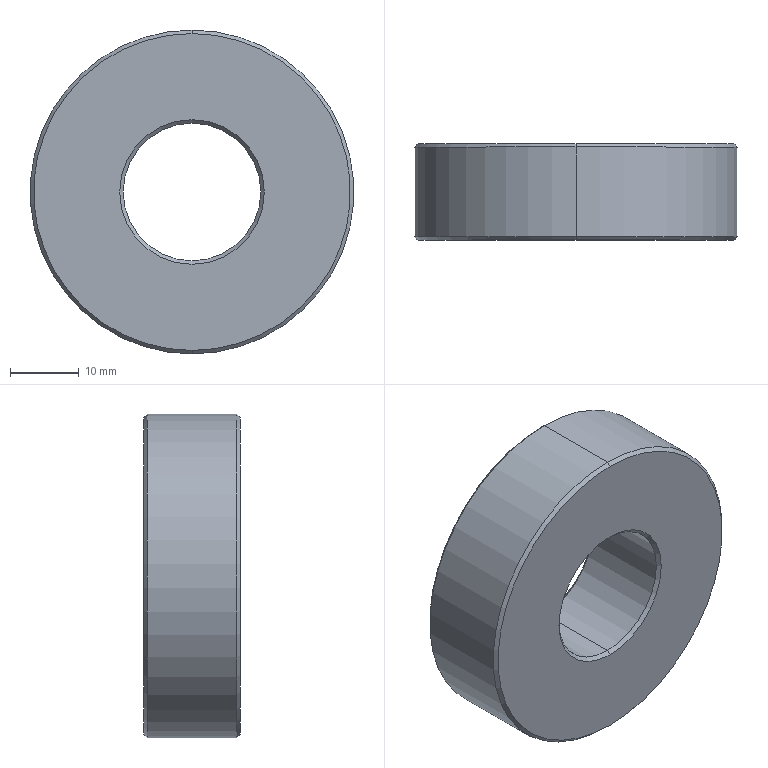Part | SolidWorks | features Chamfer 1, Extrusion 1 | 1 solid | 14 faces | box 47 x 14 x 47 mm | volume 19838 mm3 | cone 8 | cylinder 4 | plane 2 | commonest cylinder face diameters 20 x2 47 x2
STEP:
#1=CARTESIAN_POINT('',(0.,13.5,-10.));
#2=VERTEX_POINT('',#1);
#3=CARTESIAN_POINT('',(0.,13.5,10.));
#4=VERTEX_POINT('',#3);
#5=CARTESIAN_POINT('',(0.,13.5,0.));
#6=DIRECTION('',(0.,1.,0.));
#7=DIRECTION('',(0.,0.,1.));
#8=AXIS2_PLACEMENT_3D('',#5,#6,#7);
#9=CIRCLE('',#8,10.);
#10=EDGE_CURVE('',#2,#4,#9,.T.);
#11=ORIENTED_EDGE('',*,*,#10,.F.);
#12=CARTESIAN_POINT('',(0.,14.,-10.5));
#13=VERTEX_POINT('',#12);
#14=CARTESIAN_POINT('',(0.,13.5,-10.));
#15=DIRECTION('',(0.,0.7071,-0.7071));
#16=VECTOR('',#15,1000.);
#17=LINE('',#14,#16);
#18=EDGE_CURVE('',#2,#13,#17,.T.);
#19=ORIENTED_EDGE('',*,*,#18,.T.);
#20=CARTESIAN_POINT('',(0.,14.,10.5));
#21=VERTEX_POINT('',#20);
#22=CARTESIAN_POINT('',(0.,14.,0.));
#23=DIRECTION('',(0.,-1.,0.));
#24=DIRECTION('',(0.,0.,1.));
#25=AXIS2_PLACEMENT_3D('',#22,#23,#24);
#26=CIRCLE('',#25,10.5);
#27=EDGE_CURVE('',#21,#13,#26,.T.);
#28=ORIENTED_EDGE('',*,*,#27,.F.);
#29=CARTESIAN_POINT('',(0.,13.5,10.));
#30=DIRECTION('',(0.,0.7071,0.7071));
#31=VECTOR('',#30,1000.);
#32=LINE('',#29,#31);
#33=EDGE_CURVE('',#4,#21,#32,.T.);
#34=ORIENTED_EDGE('',*,*,#33,.F.);
#35=EDGE_LOOP('',(#11,#19,#28,#34));
#36=FACE_OUTER_BOUND('',#35,.T.);
#37=CARTESIAN_POINT('',(0.,13.5,0.));
#38=DIRECTION('',(0.,1.,0.));
#39=DIRECTION('',(0.,0.,1.));
#40=AXIS2_PLACEMENT_3D('',#37,#38,#39);
#41=CONICAL_SURFACE('',#40,10.,0.7854);
#42=ADVANCED_FACE('',(#36),#41,.F.);
#43=CARTESIAN_POINT('',(0.,14.,23.));
#44=VERTEX_POINT('',#43);
#45=CARTESIAN_POINT('',(0.,14.,-23.));
#46=VERTEX_POINT('',#45);
#47=CARTESIAN_POINT('',(0.,14.,0.));
#48=DIRECTION('',(0.,1.,0.));
#49=DIRECTION('',(0.,0.,1.));
#50=AXIS2_PLACEMENT_3D('',#47,#48,#49);
#51=CIRCLE('',#50,23.);
#52=EDGE_CURVE('',#44,#46,#51,.T.);
#53=ORIENTED_EDGE('',*,*,#52,.F.);
#54=CARTESIAN_POINT('',(0.,13.5,23.5));
#55=VERTEX_POINT('',#54);
#56=CARTESIAN_POINT('',(0.,14.,23.));
#57=DIRECTION('',(0.,-0.7071,0.7071));
#58=VECTOR('',#57,1000.);
#59=LINE('',#56,#58);
#60=EDGE_CURVE('',#44,#55,#59,.T.);
#61=ORIENTED_EDGE('',*,*,#60,.T.);
#62=CARTESIAN_POINT('',(0.,13.5,-23.5));
#63=VERTEX_POINT('',#62);
#64=CARTESIAN_POINT('',(0.,13.5,0.));
#65=DIRECTION('',(0.,-1.,0.));
#66=DIRECTION('',(0.,0.,1.));
#67=AXIS2_PLACEMENT_3D('',#64,#65,#66);
#68=CIRCLE('',#67,23.5);
#69=EDGE_CURVE('',#63,#55,#68,.T.);
#70=ORIENTED_EDGE('',*,*,#69,.F.);
#71=CARTESIAN_POINT('',(0.,14.,-23.));
#72=DIRECTION('',(0.,-0.7071,-0.7071));
#73=VECTOR('',#72,1000.);
#74=LINE('',#71,#73);
#75=EDGE_CURVE('',#46,#63,#74,.T.);
#76=ORIENTED_EDGE('',*,*,#75,.F.);
#77=EDGE_LOOP('',(#53,#61,#70,#76));
#78=FACE_OUTER_BOUND('',#77,.T.);
#79=CARTESIAN_POINT('',(0.,14.,0.));
#80=DIRECTION('',(0.,-1.,0.));
#81=DIRECTION('',(0.,0.,-1.));
#82=AXIS2_PLACEMENT_3D('',#79,#80,#81);
#83=CONICAL_SURFACE('',#82,23.,0.7854);
#84=ADVANCED_FACE('',(#78),#83,.T.);
#85=CARTESIAN_POINT('',(0.,0.,-23.));
#86=VERTEX_POINT('',#85);
#87=CARTESIAN_POINT('',(0.,0.,23.));
#88=VERTEX_POINT('',#87);
#89=CARTESIAN_POINT('',(0.,0.,0.));
#90=DIRECTION('',(0.,-1.,0.));
#91=DIRECTION('',(0.,0.,1.));
#92=AXIS2_PLACEMENT_3D('',#89,#90,#91);
#93=CIRCLE('',#92,23.);
#94=EDGE_CURVE('',#86,#88,#93,.T.);
#95=ORIENTED_EDGE('',*,*,#94,.F.);
#96=CARTESIAN_POINT('',(0.,0.5,-23.5));
#97=VERTEX_POINT('',#96);
#98=CARTESIAN_POINT('',(0.,0.5,-23.5));
#99=DIRECTION('',(0.,0.7071,-0.7071));
#100=VECTOR('',#99,1000.);
#101=LINE('',#98,#100);
#102=EDGE_CURVE('',#86,#97,#101,.T.);
#103=ORIENTED_EDGE('',*,*,#102,.T.);
#104=CARTESIAN_POINT('',(0.,0.5,23.5));
#105=VERTEX_POINT('',#104);
#106=CARTESIAN_POINT('',(0.,0.5,0.));
#107=DIRECTION('',(0.,1.,0.));
#108=DIRECTION('',(0.,0.,1.));
#109=AXIS2_PLACEMENT_3D('',#106,#107,#108);
#110=CIRCLE('',#109,23.5);
#111=EDGE_CURVE('',#105,#97,#110,.T.);
#112=ORIENTED_EDGE('',*,*,#111,.F.);
#113=CARTESIAN_POINT('',(0.,0.5,23.5));
#114=DIRECTION('',(0.,0.7071,0.7071));
#115=VECTOR('',#114,1000.);
#116=LINE('',#113,#115);
#117=EDGE_CURVE('',#88,#105,#116,.T.);
#118=ORIENTED_EDGE('',*,*,#117,.F.);
#119=EDGE_LOOP('',(#95,#103,#112,#118));
#120=FACE_OUTER_BOUND('',#119,.T.);
#121=CARTESIAN_POINT('',(0.,0.5,0.));
#122=DIRECTION('',(0.,1.,0.));
#123=DIRECTION('',(0.,0.,1.));
#124=AXIS2_PLACEMENT_3D('',#121,#122,#123);
#125=CONICAL_SURFACE('',#124,23.5,0.7854);
#126=ADVANCED_FACE('',(#120),#125,.T.);
#127=CARTESIAN_POINT('',(0.,0.5,10.));
#128=VERTEX_POINT('',#127);
#129=CARTESIAN_POINT('',(0.,0.5,-10.));
#130=VERTEX_POINT('',#129);
#131=CARTESIAN_POINT('',(0.,0.5,0.));
#132=DIRECTION('',(0.,-1.,0.));
#133=DIRECTION('',(0.,0.,1.));
#134=AXIS2_PLACEMENT_3D('',#131,#132,#133);
#135=CIRCLE('',#134,10.);
#136=EDGE_CURVE('',#128,#130,#135,.T.);
#137=ORIENTED_EDGE('',*,*,#136,.F.);
#138=CARTESIAN_POINT('',(0.,0.,10.5));
#139=VERTEX_POINT('',#138);
#140=CARTESIAN_POINT('',(0.,0.,10.5));
#141=DIRECTION('',(0.,-0.7071,0.7071));
#142=VECTOR('',#141,1000.);
#143=LINE('',#140,#142);
#144=EDGE_CURVE('',#128,#139,#143,.T.);
#145=ORIENTED_EDGE('',*,*,#144,.T.);
#146=CARTESIAN_POINT('',(0.,0.,-10.5));
#147=VERTEX_POINT('',#146);
#148=CARTESIAN_POINT('',(0.,0.,0.));
#149=DIRECTION('',(0.,1.,0.));
#150=DIRECTION('',(0.,0.,1.));
#151=AXIS2_PLACEMENT_3D('',#148,#149,#150);
#152=CIRCLE('',#151,10.5);
#153=EDGE_CURVE('',#147,#139,#152,.T.);
#154=ORIENTED_EDGE('',*,*,#153,.F.);
#155=CARTESIAN_POINT('',(0.,0.,-10.5));
#156=DIRECTION('',(0.,-0.7071,-0.7071));
#157=VECTOR('',#156,1000.);
#158=LINE('',#155,#157);
#159=EDGE_CURVE('',#130,#147,#158,.T.);
#160=ORIENTED_EDGE('',*,*,#159,.F.);
#161=EDGE_LOOP('',(#137,#145,#154,#160));
#162=FACE_OUTER_BOUND('',#161,.T.);
#163=CARTESIAN_POINT('',(0.,0.,0.));
#164=DIRECTION('',(0.,-1.,0.));
#165=DIRECTION('',(0.,0.,-1.));
#166=AXIS2_PLACEMENT_3D('',#163,#164,#165);
#167=CONICAL_SURFACE('',#166,10.5,0.7854);
#168=ADVANCED_FACE('',(#162),#167,.F.);
#169=ORIENTED_EDGE('',*,*,#10,.T.);
#170=CARTESIAN_POINT('',(0.,14.,10.));
#171=DIRECTION('',(0.,-1.,0.));
#172=VECTOR('',#171,1000.);
#173=LINE('',#170,#172);
#174=EDGE_CURVE('',#4,#128,#173,.T.);
#175=ORIENTED_EDGE('',*,*,#174,.T.);
#176=ORIENTED_EDGE('',*,*,#136,.T.);
#177=CARTESIAN_POINT('',(0.,14.,-10.));
#178=DIRECTION('',(0.,-1.,0.));
#179=VECTOR('',#178,1000.);
#180=LINE('',#177,#179);
#181=EDGE_CURVE('',#2,#130,#180,.T.);
#182=ORIENTED_EDGE('',*,*,#181,.F.);
#183=EDGE_LOOP('',(#169,#175,#176,#182));
#184=FACE_OUTER_BOUND('',#183,.T.);
#185=CARTESIAN_POINT('',(0.,14.,0.));
#186=DIRECTION('',(0.,-1.,0.));
#187=DIRECTION('',(0.,0.,-1.));
#188=AXIS2_PLACEMENT_3D('',#185,#186,#187);
#189=CYLINDRICAL_SURFACE('',#188,10.);
#190=ADVANCED_FACE('',(#184),#189,.F.);
#191=ORIENTED_EDGE('',*,*,#69,.T.);
#192=CARTESIAN_POINT('',(0.,14.,23.5));
#193=DIRECTION('',(0.,-1.,0.));
#194=VECTOR('',#193,1000.);
#195=LINE('',#192,#194);
#196=EDGE_CURVE('',#55,#105,#195,.T.);
#197=ORIENTED_EDGE('',*,*,#196,.T.);
#198=ORIENTED_EDGE('',*,*,#111,.T.);
#199=CARTESIAN_POINT('',(0.,14.,-23.5));
#200=DIRECTION('',(0.,-1.,0.));
#201=VECTOR('',#200,1000.);
#202=LINE('',#199,#201);
#203=EDGE_CURVE('',#63,#97,#202,.T.);
#204=ORIENTED_EDGE('',*,*,#203,.F.);
#205=EDGE_LOOP('',(#191,#197,#198,#204));
#206=FACE_OUTER_BOUND('',#205,.T.);
#207=CARTESIAN_POINT('',(0.,14.,0.));
#208=DIRECTION('',(0.,-1.,0.));
#209=DIRECTION('',(0.,0.,-1.));
#210=AXIS2_PLACEMENT_3D('',#207,#208,#209);
#211=CYLINDRICAL_SURFACE('',#210,23.5);
#212=ADVANCED_FACE('',(#206),#211,.T.);
#213=CARTESIAN_POINT('',(0.,14.,0.));
#214=DIRECTION('',(0.,1.,0.));
#215=DIRECTION('',(0.,0.,1.));
#216=AXIS2_PLACEMENT_3D('',#213,#214,#215);
#217=CIRCLE('',#216,23.);
#218=EDGE_CURVE('',#46,#44,#217,.T.);
#219=ORIENTED_EDGE('',*,*,#218,.T.);
#220=ORIENTED_EDGE('',*,*,#52,.T.);
#221=EDGE_LOOP('',(#219,#220));
#222=FACE_OUTER_BOUND('',#221,.T.);
#223=ORIENTED_EDGE('',*,*,#27,.T.);
#224=CARTESIAN_POINT('',(0.,14.,0.));
#225=DIRECTION('',(0.,-1.,0.));
#226=DIRECTION('',(0.,0.,1.));
#227=AXIS2_PLACEMENT_3D('',#224,#225,#226);
#228=CIRCLE('',#227,10.5);
#229=EDGE_CURVE('',#13,#21,#228,.T.);
#230=ORIENTED_EDGE('',*,*,#229,.T.);
#231=EDGE_LOOP('',(#223,#230));
#232=FACE_BOUND('',#231,.T.);
#233=CARTESIAN_POINT('',(0.,14.,0.));
#234=DIRECTION('',(0.,1.,0.));
#235=DIRECTION('',(0.,0.,1.));
#236=AXIS2_PLACEMENT_3D('',#233,#234,#235);
#237=PLANE('',#236);
#238=ADVANCED_FACE('',(#222,#232),#237,.T.);
#239=ORIENTED_EDGE('',*,*,#153,.T.);
#240=CARTESIAN_POINT('',(0.,0.,0.));
#241=DIRECTION('',(0.,1.,0.));
#242=DIRECTION('',(0.,0.,1.));
#243=AXIS2_PLACEMENT_3D('',#240,#241,#242);
#244=CIRCLE('',#243,10.5);
#245=EDGE_CURVE('',#139,#147,#244,.T.);
#246=ORIENTED_EDGE('',*,*,#245,.T.);
#247=EDGE_LOOP('',(#239,#246));
#248=FACE_BOUND('',#247,.T.);
#249=CARTESIAN_POINT('',(0.,0.,0.));
#250=DIRECTION('',(0.,-1.,0.));
#251=DIRECTION('',(0.,0.,1.));
#252=AXIS2_PLACEMENT_3D('',#249,#250,#251);
#253=CIRCLE('',#252,23.);
#254=EDGE_CURVE('',#88,#86,#253,.T.);
#255=ORIENTED_EDGE('',*,*,#254,.T.);
#256=ORIENTED_EDGE('',*,*,#94,.T.);
#257=EDGE_LOOP('',(#255,#256));
#258=FACE_OUTER_BOUND('',#257,.T.);
#259=CARTESIAN_POINT('',(0.,0.,0.));
#260=DIRECTION('',(0.,1.,0.));
#261=DIRECTION('',(0.,0.,1.));
#262=AXIS2_PLACEMENT_3D('',#259,#260,#261);
#263=PLANE('',#262);
#264=ADVANCED_FACE('',(#248,#258),#263,.F.);
#265=ORIENTED_EDGE('',*,*,#196,.F.);
#266=CARTESIAN_POINT('',(0.,13.5,0.));
#267=DIRECTION('',(0.,-1.,0.));
#268=DIRECTION('',(0.,0.,1.));
#269=AXIS2_PLACEMENT_3D('',#266,#267,#268);
#270=CIRCLE('',#269,23.5);
#271=EDGE_CURVE('',#55,#63,#270,.T.);
#272=ORIENTED_EDGE('',*,*,#271,.T.);
#273=ORIENTED_EDGE('',*,*,#203,.T.);
#274=CARTESIAN_POINT('',(0.,0.5,0.));
#275=DIRECTION('',(0.,1.,0.));
#276=DIRECTION('',(0.,0.,1.));
#277=AXIS2_PLACEMENT_3D('',#274,#275,#276);
#278=CIRCLE('',#277,23.5);
#279=EDGE_CURVE('',#97,#105,#278,.T.);
#280=ORIENTED_EDGE('',*,*,#279,.T.);
#281=EDGE_LOOP('',(#265,#272,#273,#280));
#282=FACE_OUTER_BOUND('',#281,.T.);
#283=CARTESIAN_POINT('',(0.,14.,0.));
#284=DIRECTION('',(0.,-1.,0.));
#285=DIRECTION('',(0.,0.,-1.));
#286=AXIS2_PLACEMENT_3D('',#283,#284,#285);
#287=CYLINDRICAL_SURFACE('',#286,23.5);
#288=ADVANCED_FACE('',(#282),#287,.T.);
#289=ORIENTED_EDGE('',*,*,#174,.F.);
#290=CARTESIAN_POINT('',(0.,13.5,0.));
#291=DIRECTION('',(0.,1.,0.));
#292=DIRECTION('',(0.,0.,1.));
#293=AXIS2_PLACEMENT_3D('',#290,#291,#292);
#294=CIRCLE('',#293,10.);
#295=EDGE_CURVE('',#4,#2,#294,.T.);
#296=ORIENTED_EDGE('',*,*,#295,.T.);
#297=ORIENTED_EDGE('',*,*,#181,.T.);
#298=CARTESIAN_POINT('',(0.,0.5,0.));
#299=DIRECTION('',(0.,-1.,0.));
#300=DIRECTION('',(0.,0.,1.));
#301=AXIS2_PLACEMENT_3D('',#298,#299,#300);
#302=CIRCLE('',#301,10.);
#303=EDGE_CURVE('',#130,#128,#302,.T.);
#304=ORIENTED_EDGE('',*,*,#303,.T.);
#305=EDGE_LOOP('',(#289,#296,#297,#304));
#306=FACE_OUTER_BOUND('',#305,.T.);
#307=CARTESIAN_POINT('',(0.,14.,0.));
#308=DIRECTION('',(0.,-1.,0.));
#309=DIRECTION('',(0.,0.,-1.));
#310=AXIS2_PLACEMENT_3D('',#307,#308,#309);
#311=CYLINDRICAL_SURFACE('',#310,10.);
#312=ADVANCED_FACE('',(#306),#311,.F.);
#313=ORIENTED_EDGE('',*,*,#144,.F.);
#314=ORIENTED_EDGE('',*,*,#303,.F.);
#315=ORIENTED_EDGE('',*,*,#159,.T.);
#316=ORIENTED_EDGE('',*,*,#245,.F.);
#317=EDGE_LOOP('',(#313,#314,#315,#316));
#318=FACE_OUTER_BOUND('',#317,.T.);
#319=CARTESIAN_POINT('',(0.,0.,0.));
#320=DIRECTION('',(0.,-1.,0.));
#321=DIRECTION('',(0.,0.,-1.));
#322=AXIS2_PLACEMENT_3D('',#319,#320,#321);
#323=CONICAL_SURFACE('',#322,10.5,0.7854);
#324=ADVANCED_FACE('',(#318),#323,.F.);
#325=ORIENTED_EDGE('',*,*,#102,.F.);
#326=ORIENTED_EDGE('',*,*,#254,.F.);
#327=ORIENTED_EDGE('',*,*,#117,.T.);
#328=ORIENTED_EDGE('',*,*,#279,.F.);
#329=EDGE_LOOP('',(#325,#326,#327,#328));
#330=FACE_OUTER_BOUND('',#329,.T.);
#331=CARTESIAN_POINT('',(0.,0.5,0.));
#332=DIRECTION('',(0.,1.,0.));
#333=DIRECTION('',(0.,0.,1.));
#334=AXIS2_PLACEMENT_3D('',#331,#332,#333);
#335=CONICAL_SURFACE('',#334,23.5,0.7854);
#336=ADVANCED_FACE('',(#330),#335,.T.);
#337=ORIENTED_EDGE('',*,*,#60,.F.);
#338=ORIENTED_EDGE('',*,*,#218,.F.);
#339=ORIENTED_EDGE('',*,*,#75,.T.);
#340=ORIENTED_EDGE('',*,*,#271,.F.);
#341=EDGE_LOOP('',(#337,#338,#339,#340));
#342=FACE_OUTER_BOUND('',#341,.T.);
#343=CARTESIAN_POINT('',(0.,14.,0.));
#344=DIRECTION('',(0.,-1.,0.));
#345=DIRECTION('',(0.,0.,-1.));
#346=AXIS2_PLACEMENT_3D('',#343,#344,#345);
#347=CONICAL_SURFACE('',#346,23.,0.7854);
#348=ADVANCED_FACE('',(#342),#347,.T.);
#349=ORIENTED_EDGE('',*,*,#18,.F.);
#350=ORIENTED_EDGE('',*,*,#295,.F.);
#351=ORIENTED_EDGE('',*,*,#33,.T.);
#352=ORIENTED_EDGE('',*,*,#229,.F.);
#353=EDGE_LOOP('',(#349,#350,#351,#352));
#354=FACE_OUTER_BOUND('',#353,.T.);
#355=CARTESIAN_POINT('',(0.,13.5,0.));
#356=DIRECTION('',(0.,1.,0.));
#357=DIRECTION('',(0.,0.,1.));
#358=AXIS2_PLACEMENT_3D('',#355,#356,#357);
#359=CONICAL_SURFACE('',#358,10.,0.7854);
#360=ADVANCED_FACE('',(#354),#359,.F.);
#361=CLOSED_SHELL('',(#42,#84,#126,#168,#190,#212,#238,#264,#288,#312,#324,#336,#348,#360));
#362=MANIFOLD_SOLID_BREP('',#361);
#363=CARTESIAN_POINT('',(0.,0.,0.));
#364=DIRECTION('',(0.,0.,1.));
#365=DIRECTION('',(1.,0.,0.));
#366=AXIS2_PLACEMENT_3D('',#363,#364,#365);
#367=(LENGTH_UNIT()NAMED_UNIT(*)SI_UNIT(.MILLI.,.METRE.));
#368=UNCERTAINTY_MEASURE_WITH_UNIT(LENGTH_MEASURE(0.00001),#367,'','');
#369=(NAMED_UNIT(*)PLANE_ANGLE_UNIT()SI_UNIT($,.RADIAN.));
#370=(NAMED_UNIT(*)SI_UNIT($,.STERADIAN.)SOLID_ANGLE_UNIT());
#371=(GEOMETRIC_REPRESENTATION_CONTEXT(3)GLOBAL_UNCERTAINTY_ASSIGNED_CONTEXT((#368))GLOBAL_UNIT_ASSIGNED_CONTEXT((#367,#369,#370))REPRESENTATION_CONTEXT('',''));
#372=ADVANCED_BREP_SHAPE_REPRESENTATION('',(#362,#366),#371);